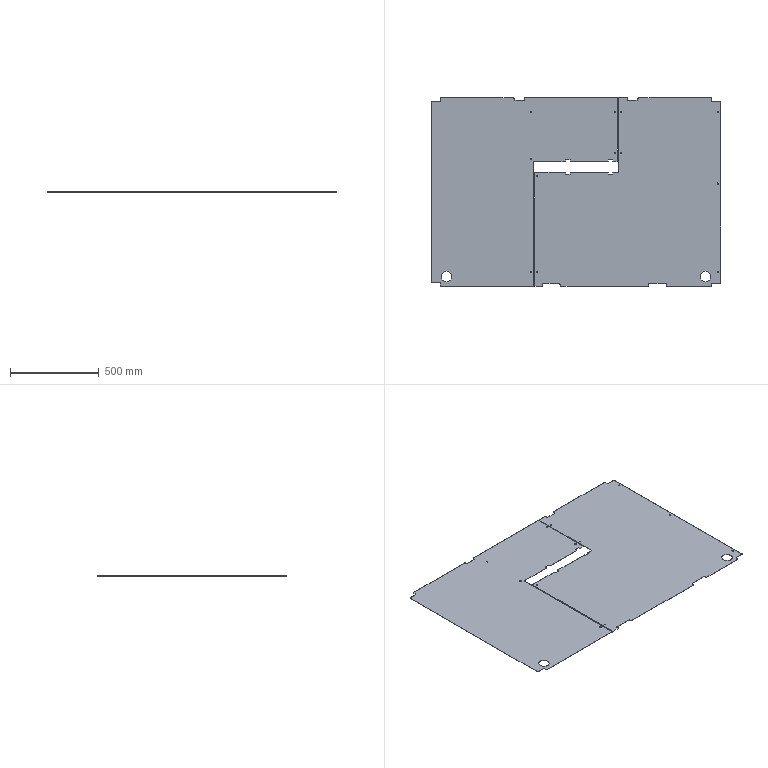Part | SolidWorks | features ICE 9, Fillet 5, FlatPattern 2, HoleWzd 1, SMBaseFlange 1, SheetMetal 1 | 2 solids | 128 faces | box 1632 x 1065 x 1.2 mm | volume 2027394 mm3 | cylinder 72 | plane 56 | commonest cylinder face diameters 10 x29 7 x24 6 x15 59 x4